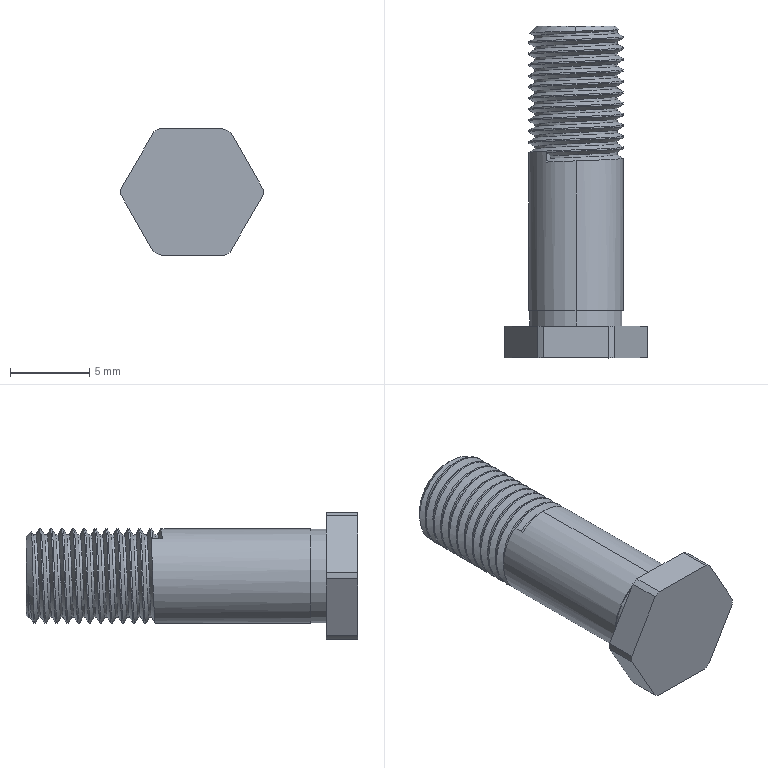Part | NX | features BREP 1 | 1 solid | 49 faces | box 9 x 21 x 8.027 mm | volume 612.415 mm3 | cylinder 33 | plane 11 | cone 3 | spline 2 | commonest cylinder face diameters 6 x24 9 x6 5.9 x2 5.242 x1